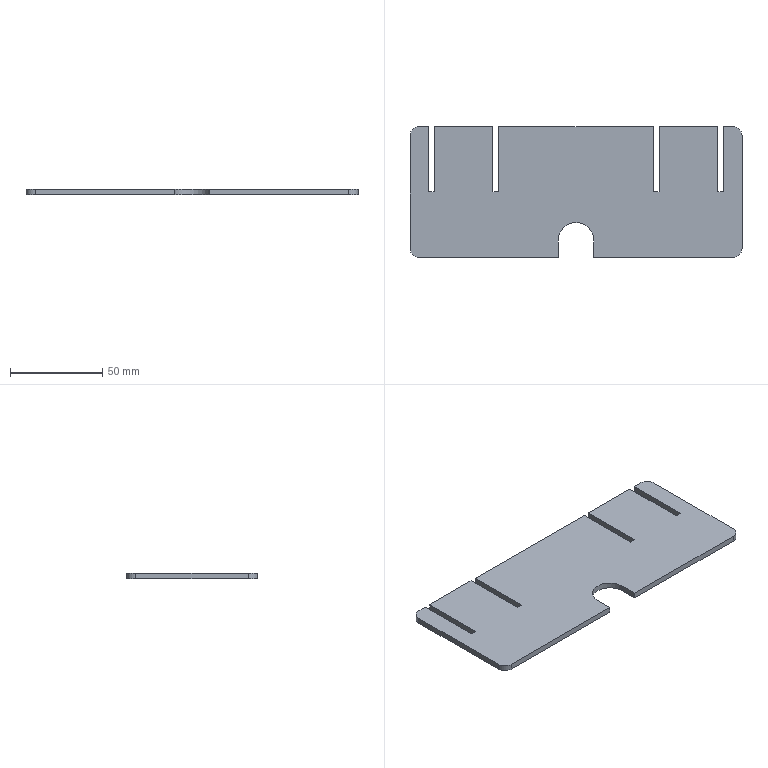Part | SolidWorks | features FlatPattern 1, SMBaseFlange 1, SheetMetal 1 | 1 solid | 30 faces | box 180 x 71 x 3.2 mm | volume 38342 mm3 | plane 25 | cylinder 5 | commonest cylinder face diameters 10 x4 19 x1
STEP:
#1=CARTESIAN_POINT('',(-146.71,-88.278,0.));
#2=VERTEX_POINT('',#1);
#3=CARTESIAN_POINT('',(-151.71,-88.278,0.));
#4=VERTEX_POINT('',#3);
#5=CARTESIAN_POINT('',(-146.71,-88.278,0.));
#6=DIRECTION('',(-1.,0.,0.));
#7=VECTOR('',#6,1000.);
#8=LINE('',#5,#7);
#9=EDGE_CURVE('',#2,#4,#8,.T.);
#10=ORIENTED_EDGE('',*,*,#9,.F.);
#11=CARTESIAN_POINT('',(-146.71,-88.278,-3.2));
#12=VERTEX_POINT('',#11);
#13=CARTESIAN_POINT('',(-146.71,-88.278,-3.2));
#14=DIRECTION('',(0.,0.,1.));
#15=VECTOR('',#14,1000.);
#16=LINE('',#13,#15);
#17=EDGE_CURVE('',#12,#2,#16,.T.);
#18=ORIENTED_EDGE('',*,*,#17,.F.);
#19=CARTESIAN_POINT('',(-151.71,-88.278,-3.2));
#20=VERTEX_POINT('',#19);
#21=CARTESIAN_POINT('',(-146.71,-88.278,-3.2));
#22=DIRECTION('',(-1.,0.,0.));
#23=VECTOR('',#22,1000.);
#24=LINE('',#21,#23);
#25=EDGE_CURVE('',#12,#20,#24,.T.);
#26=ORIENTED_EDGE('',*,*,#25,.T.);
#27=CARTESIAN_POINT('',(-151.71,-88.278,-3.2));
#28=DIRECTION('',(0.,0.,1.));
#29=VECTOR('',#28,1000.);
#30=LINE('',#27,#29);
#31=EDGE_CURVE('',#20,#4,#30,.T.);
#32=ORIENTED_EDGE('',*,*,#31,.T.);
#33=EDGE_LOOP('',(#10,#18,#26,#32));
#34=FACE_OUTER_BOUND('',#33,.T.);
#35=CARTESIAN_POINT('',(-146.71,-88.278,-3.2));
#36=DIRECTION('',(0.,1.,0.));
#37=DIRECTION('',(-1.,0.,0.));
#38=AXIS2_PLACEMENT_3D('',#35,#36,#37);
#39=PLANE('',#38);
#40=ADVANCED_FACE('',(#34),#39,.T.);
#41=CARTESIAN_POINT('',(-146.71,-123.778,0.));
#42=VERTEX_POINT('',#41);
#43=CARTESIAN_POINT('',(-146.71,-88.278,0.));
#44=DIRECTION('',(0.,1.,0.));
#45=VECTOR('',#44,1000.);
#46=LINE('',#43,#45);
#47=EDGE_CURVE('',#42,#2,#46,.T.);
#48=ORIENTED_EDGE('',*,*,#47,.F.);
#49=CARTESIAN_POINT('',(-146.71,-123.778,-3.2));
#50=VERTEX_POINT('',#49);
#51=CARTESIAN_POINT('',(-146.71,-123.778,-3.2));
#52=DIRECTION('',(0.,0.,1.));
#53=VECTOR('',#52,1000.);
#54=LINE('',#51,#53);
#55=EDGE_CURVE('',#50,#42,#54,.T.);
#56=ORIENTED_EDGE('',*,*,#55,.F.);
#57=CARTESIAN_POINT('',(-146.71,-88.278,-3.2));
#58=DIRECTION('',(0.,1.,0.));
#59=VECTOR('',#58,1000.);
#60=LINE('',#57,#59);
#61=EDGE_CURVE('',#50,#12,#60,.T.);
#62=ORIENTED_EDGE('',*,*,#61,.T.);
#63=ORIENTED_EDGE('',*,*,#17,.T.);
#64=EDGE_LOOP('',(#48,#56,#62,#63));
#65=FACE_OUTER_BOUND('',#64,.T.);
#66=CARTESIAN_POINT('',(-146.71,-88.278,-3.2));
#67=DIRECTION('',(1.,0.,0.));
#68=DIRECTION('',(0.,1.,0.));
#69=AXIS2_PLACEMENT_3D('',#66,#67,#68);
#70=PLANE('',#69);
#71=ADVANCED_FACE('',(#65),#70,.T.);
#72=CARTESIAN_POINT('',(-143.51,-123.778,0.));
#73=VERTEX_POINT('',#72);
#74=CARTESIAN_POINT('',(-146.71,-123.778,0.));
#75=DIRECTION('',(-1.,0.,0.));
#76=VECTOR('',#75,1000.);
#77=LINE('',#74,#76);
#78=EDGE_CURVE('',#73,#42,#77,.T.);
#79=ORIENTED_EDGE('',*,*,#78,.F.);
#80=CARTESIAN_POINT('',(-143.51,-123.778,-3.2));
#81=VERTEX_POINT('',#80);
#82=CARTESIAN_POINT('',(-143.51,-123.778,-3.2));
#83=DIRECTION('',(0.,0.,1.));
#84=VECTOR('',#83,1000.);
#85=LINE('',#82,#84);
#86=EDGE_CURVE('',#81,#73,#85,.T.);
#87=ORIENTED_EDGE('',*,*,#86,.F.);
#88=CARTESIAN_POINT('',(-146.71,-123.778,-3.2));
#89=DIRECTION('',(-1.,0.,0.));
#90=VECTOR('',#89,1000.);
#91=LINE('',#88,#90);
#92=EDGE_CURVE('',#81,#50,#91,.T.);
#93=ORIENTED_EDGE('',*,*,#92,.T.);
#94=ORIENTED_EDGE('',*,*,#55,.T.);
#95=EDGE_LOOP('',(#79,#87,#93,#94));
#96=FACE_OUTER_BOUND('',#95,.T.);
#97=CARTESIAN_POINT('',(-146.71,-123.778,-3.2));
#98=DIRECTION('',(0.,1.,0.));
#99=DIRECTION('',(0.,0.,1.));
#100=AXIS2_PLACEMENT_3D('',#97,#98,#99);
#101=PLANE('',#100);
#102=ADVANCED_FACE('',(#96),#101,.T.);
#103=CARTESIAN_POINT('',(-143.51,-88.278,0.));
#104=VERTEX_POINT('',#103);
#105=CARTESIAN_POINT('',(-143.51,-123.778,0.));
#106=DIRECTION('',(0.,-1.,0.));
#107=VECTOR('',#106,1000.);
#108=LINE('',#105,#107);
#109=EDGE_CURVE('',#104,#73,#108,.T.);
#110=ORIENTED_EDGE('',*,*,#109,.F.);
#111=CARTESIAN_POINT('',(-143.51,-88.278,-3.2));
#112=VERTEX_POINT('',#111);
#113=CARTESIAN_POINT('',(-143.51,-88.278,-3.2));
#114=DIRECTION('',(0.,0.,1.));
#115=VECTOR('',#114,1000.);
#116=LINE('',#113,#115);
#117=EDGE_CURVE('',#112,#104,#116,.T.);
#118=ORIENTED_EDGE('',*,*,#117,.F.);
#119=CARTESIAN_POINT('',(-143.51,-123.778,-3.2));
#120=DIRECTION('',(0.,-1.,0.));
#121=VECTOR('',#120,1000.);
#122=LINE('',#119,#121);
#123=EDGE_CURVE('',#112,#81,#122,.T.);
#124=ORIENTED_EDGE('',*,*,#123,.T.);
#125=ORIENTED_EDGE('',*,*,#86,.T.);
#126=EDGE_LOOP('',(#110,#118,#124,#125));
#127=FACE_OUTER_BOUND('',#126,.T.);
#128=CARTESIAN_POINT('',(-143.51,-123.778,-3.2));
#129=DIRECTION('',(-1.,0.,0.));
#130=DIRECTION('',(0.,-1.,0.));
#131=AXIS2_PLACEMENT_3D('',#128,#129,#130);
#132=PLANE('',#131);
#133=ADVANCED_FACE('',(#127),#132,.T.);
#134=CARTESIAN_POINT('',(-111.71,-88.278,0.));
#135=VERTEX_POINT('',#134);
#136=CARTESIAN_POINT('',(-111.71,-88.278,0.));
#137=DIRECTION('',(-1.,0.,0.));
#138=VECTOR('',#137,1000.);
#139=LINE('',#136,#138);
#140=EDGE_CURVE('',#135,#104,#139,.T.);
#141=ORIENTED_EDGE('',*,*,#140,.F.);
#142=CARTESIAN_POINT('',(-111.71,-88.278,-3.2));
#143=VERTEX_POINT('',#142);
#144=CARTESIAN_POINT('',(-111.71,-88.278,-3.2));
#145=DIRECTION('',(0.,0.,1.));
#146=VECTOR('',#145,1000.);
#147=LINE('',#144,#146);
#148=EDGE_CURVE('',#143,#135,#147,.T.);
#149=ORIENTED_EDGE('',*,*,#148,.F.);
#150=CARTESIAN_POINT('',(-111.71,-88.278,-3.2));
#151=DIRECTION('',(-1.,0.,0.));
#152=VECTOR('',#151,1000.);
#153=LINE('',#150,#152);
#154=EDGE_CURVE('',#143,#112,#153,.T.);
#155=ORIENTED_EDGE('',*,*,#154,.T.);
#156=ORIENTED_EDGE('',*,*,#117,.T.);
#157=EDGE_LOOP('',(#141,#149,#155,#156));
#158=FACE_OUTER_BOUND('',#157,.T.);
#159=CARTESIAN_POINT('',(-111.71,-88.278,-3.2));
#160=DIRECTION('',(0.,1.,0.));
#161=DIRECTION('',(-1.,0.,0.));
#162=AXIS2_PLACEMENT_3D('',#159,#160,#161);
#163=PLANE('',#162);
#164=ADVANCED_FACE('',(#158),#163,.T.);
#165=CARTESIAN_POINT('',(-111.71,-123.778,0.));
#166=VERTEX_POINT('',#165);
#167=CARTESIAN_POINT('',(-111.71,-88.278,0.));
#168=DIRECTION('',(0.,1.,0.));
#169=VECTOR('',#168,1000.);
#170=LINE('',#167,#169);
#171=EDGE_CURVE('',#166,#135,#170,.T.);
#172=ORIENTED_EDGE('',*,*,#171,.F.);
#173=CARTESIAN_POINT('',(-111.71,-123.778,-3.2));
#174=VERTEX_POINT('',#173);
#175=CARTESIAN_POINT('',(-111.71,-123.778,-3.2));
#176=DIRECTION('',(0.,0.,1.));
#177=VECTOR('',#176,1000.);
#178=LINE('',#175,#177);
#179=EDGE_CURVE('',#174,#166,#178,.T.);
#180=ORIENTED_EDGE('',*,*,#179,.F.);
#181=CARTESIAN_POINT('',(-111.71,-88.278,-3.2));
#182=DIRECTION('',(0.,1.,0.));
#183=VECTOR('',#182,1000.);
#184=LINE('',#181,#183);
#185=EDGE_CURVE('',#174,#143,#184,.T.);
#186=ORIENTED_EDGE('',*,*,#185,.T.);
#187=ORIENTED_EDGE('',*,*,#148,.T.);
#188=EDGE_LOOP('',(#172,#180,#186,#187));
#189=FACE_OUTER_BOUND('',#188,.T.);
#190=CARTESIAN_POINT('',(-111.71,-88.278,-3.2));
#191=DIRECTION('',(1.,0.,0.));
#192=DIRECTION('',(0.,1.,0.));
#193=AXIS2_PLACEMENT_3D('',#190,#191,#192);
#194=PLANE('',#193);
#195=ADVANCED_FACE('',(#189),#194,.T.);
#196=CARTESIAN_POINT('',(-108.51,-123.778,0.));
#197=VERTEX_POINT('',#196);
#198=CARTESIAN_POINT('',(-111.71,-123.778,0.));
#199=DIRECTION('',(-1.,0.,0.));
#200=VECTOR('',#199,1000.);
#201=LINE('',#198,#200);
#202=EDGE_CURVE('',#197,#166,#201,.T.);
#203=ORIENTED_EDGE('',*,*,#202,.F.);
#204=CARTESIAN_POINT('',(-108.51,-123.778,-3.2));
#205=VERTEX_POINT('',#204);
#206=CARTESIAN_POINT('',(-108.51,-123.778,-3.2));
#207=DIRECTION('',(0.,0.,1.));
#208=VECTOR('',#207,1000.);
#209=LINE('',#206,#208);
#210=EDGE_CURVE('',#205,#197,#209,.T.);
#211=ORIENTED_EDGE('',*,*,#210,.F.);
#212=CARTESIAN_POINT('',(-111.71,-123.778,-3.2));
#213=DIRECTION('',(-1.,0.,0.));
#214=VECTOR('',#213,1000.);
#215=LINE('',#212,#214);
#216=EDGE_CURVE('',#205,#174,#215,.T.);
#217=ORIENTED_EDGE('',*,*,#216,.T.);
#218=ORIENTED_EDGE('',*,*,#179,.T.);
#219=EDGE_LOOP('',(#203,#211,#217,#218));
#220=FACE_OUTER_BOUND('',#219,.T.);
#221=CARTESIAN_POINT('',(-111.71,-123.778,-3.2));
#222=DIRECTION('',(0.,1.,0.));
#223=DIRECTION('',(0.,0.,1.));
#224=AXIS2_PLACEMENT_3D('',#221,#222,#223);
#225=PLANE('',#224);
#226=ADVANCED_FACE('',(#220),#225,.T.);
#227=CARTESIAN_POINT('',(-108.51,-88.278,0.));
#228=VERTEX_POINT('',#227);
#229=CARTESIAN_POINT('',(-108.51,-123.778,0.));
#230=DIRECTION('',(0.,-1.,0.));
#231=VECTOR('',#230,1000.);
#232=LINE('',#229,#231);
#233=EDGE_CURVE('',#228,#197,#232,.T.);
#234=ORIENTED_EDGE('',*,*,#233,.F.);
#235=CARTESIAN_POINT('',(-108.51,-88.278,-3.2));
#236=VERTEX_POINT('',#235);
#237=CARTESIAN_POINT('',(-108.51,-88.278,-3.2));
#238=DIRECTION('',(0.,0.,1.));
#239=VECTOR('',#238,1000.);
#240=LINE('',#237,#239);
#241=EDGE_CURVE('',#236,#228,#240,.T.);
#242=ORIENTED_EDGE('',*,*,#241,.F.);
#243=CARTESIAN_POINT('',(-108.51,-123.778,-3.2));
#244=DIRECTION('',(0.,-1.,0.));
#245=VECTOR('',#244,1000.);
#246=LINE('',#243,#245);
#247=EDGE_CURVE('',#236,#205,#246,.T.);
#248=ORIENTED_EDGE('',*,*,#247,.T.);
#249=ORIENTED_EDGE('',*,*,#210,.T.);
#250=EDGE_LOOP('',(#234,#242,#248,#249));
#251=FACE_OUTER_BOUND('',#250,.T.);
#252=CARTESIAN_POINT('',(-108.51,-123.778,-3.2));
#253=DIRECTION('',(-1.,0.,0.));
#254=DIRECTION('',(0.,-1.,0.));
#255=AXIS2_PLACEMENT_3D('',#252,#253,#254);
#256=PLANE('',#255);
#257=ADVANCED_FACE('',(#251),#256,.T.);
#258=CARTESIAN_POINT('',(-24.91,-88.278,0.));
#259=VERTEX_POINT('',#258);
#260=CARTESIAN_POINT('',(-24.91,-88.278,0.));
#261=DIRECTION('',(-1.,0.,0.));
#262=VECTOR('',#261,1000.);
#263=LINE('',#260,#262);
#264=EDGE_CURVE('',#259,#228,#263,.T.);
#265=ORIENTED_EDGE('',*,*,#264,.F.);
#266=CARTESIAN_POINT('',(-24.91,-88.278,-3.2));
#267=VERTEX_POINT('',#266);
#268=CARTESIAN_POINT('',(-24.91,-88.278,-3.2));
#269=DIRECTION('',(0.,0.,1.));
#270=VECTOR('',#269,1000.);
#271=LINE('',#268,#270);
#272=EDGE_CURVE('',#267,#259,#271,.T.);
#273=ORIENTED_EDGE('',*,*,#272,.F.);
#274=CARTESIAN_POINT('',(-24.91,-88.278,-3.2));
#275=DIRECTION('',(-1.,0.,0.));
#276=VECTOR('',#275,1000.);
#277=LINE('',#274,#276);
#278=EDGE_CURVE('',#267,#236,#277,.T.);
#279=ORIENTED_EDGE('',*,*,#278,.T.);
#280=ORIENTED_EDGE('',*,*,#241,.T.);
#281=EDGE_LOOP('',(#265,#273,#279,#280));
#282=FACE_OUTER_BOUND('',#281,.T.);
#283=CARTESIAN_POINT('',(-24.91,-88.278,-3.2));
#284=DIRECTION('',(0.,1.,0.));
#285=DIRECTION('',(-1.,0.,0.));
#286=AXIS2_PLACEMENT_3D('',#283,#284,#285);
#287=PLANE('',#286);
#288=ADVANCED_FACE('',(#282),#287,.T.);
#289=CARTESIAN_POINT('',(-24.91,-123.778,0.));
#290=VERTEX_POINT('',#289);
#291=CARTESIAN_POINT('',(-24.91,-88.278,0.));
#292=DIRECTION('',(0.,1.,0.));
#293=VECTOR('',#292,1000.);
#294=LINE('',#291,#293);
#295=EDGE_CURVE('',#290,#259,#294,.T.);
#296=ORIENTED_EDGE('',*,*,#295,.F.);
#297=CARTESIAN_POINT('',(-24.91,-123.778,-3.2));
#298=VERTEX_POINT('',#297);
#299=CARTESIAN_POINT('',(-24.91,-123.778,-3.2));
#300=DIRECTION('',(0.,0.,1.));
#301=VECTOR('',#300,1000.);
#302=LINE('',#299,#301);
#303=EDGE_CURVE('',#298,#290,#302,.T.);
#304=ORIENTED_EDGE('',*,*,#303,.F.);
#305=CARTESIAN_POINT('',(-24.91,-88.278,-3.2));
#306=DIRECTION('',(0.,1.,0.));
#307=VECTOR('',#306,1000.);
#308=LINE('',#305,#307);
#309=EDGE_CURVE('',#298,#267,#308,.T.);
#310=ORIENTED_EDGE('',*,*,#309,.T.);
#311=ORIENTED_EDGE('',*,*,#272,.T.);
#312=EDGE_LOOP('',(#296,#304,#310,#311));
#313=FACE_OUTER_BOUND('',#312,.T.);
#314=CARTESIAN_POINT('',(-24.91,-88.278,-3.2));
#315=DIRECTION('',(1.,0.,0.));
#316=DIRECTION('',(0.,1.,0.));
#317=AXIS2_PLACEMENT_3D('',#314,#315,#316);
#318=PLANE('',#317);
#319=ADVANCED_FACE('',(#313),#318,.T.);
#320=CARTESIAN_POINT('',(-21.71,-123.778,0.));
#321=VERTEX_POINT('',#320);
#322=CARTESIAN_POINT('',(-24.91,-123.778,0.));
#323=DIRECTION('',(-1.,0.,0.));
#324=VECTOR('',#323,1000.);
#325=LINE('',#322,#324);
#326=EDGE_CURVE('',#321,#290,#325,.T.);
#327=ORIENTED_EDGE('',*,*,#326,.F.);
#328=CARTESIAN_POINT('',(-21.71,-123.778,-3.2));
#329=VERTEX_POINT('',#328);
#330=CARTESIAN_POINT('',(-21.71,-123.778,-3.2));
#331=DIRECTION('',(0.,0.,1.));
#332=VECTOR('',#331,1000.);
#333=LINE('',#330,#332);
#334=EDGE_CURVE('',#329,#321,#333,.T.);
#335=ORIENTED_EDGE('',*,*,#334,.F.);
#336=CARTESIAN_POINT('',(-24.91,-123.778,-3.2));
#337=DIRECTION('',(-1.,0.,0.));
#338=VECTOR('',#337,1000.);
#339=LINE('',#336,#338);
#340=EDGE_CURVE('',#329,#298,#339,.T.);
#341=ORIENTED_EDGE('',*,*,#340,.T.);
#342=ORIENTED_EDGE('',*,*,#303,.T.);
#343=EDGE_LOOP('',(#327,#335,#341,#342));
#344=FACE_OUTER_BOUND('',#343,.T.);
#345=CARTESIAN_POINT('',(-24.91,-123.778,-3.2));
#346=DIRECTION('',(0.,1.,0.));
#347=DIRECTION('',(0.,0.,1.));
#348=AXIS2_PLACEMENT_3D('',#345,#346,#347);
#349=PLANE('',#348);
#350=ADVANCED_FACE('',(#344),#349,.T.);
#351=CARTESIAN_POINT('',(-21.71,-88.278,0.));
#352=VERTEX_POINT('',#351);
#353=CARTESIAN_POINT('',(-21.71,-123.778,0.));
#354=DIRECTION('',(0.,-1.,0.));
#355=VECTOR('',#354,1000.);
#356=LINE('',#353,#355);
#357=EDGE_CURVE('',#352,#321,#356,.T.);
#358=ORIENTED_EDGE('',*,*,#357,.F.);
#359=CARTESIAN_POINT('',(-21.71,-88.278,-3.2));
#360=VERTEX_POINT('',#359);
#361=CARTESIAN_POINT('',(-21.71,-88.278,-3.2));
#362=DIRECTION('',(0.,0.,1.));
#363=VECTOR('',#362,1000.);
#364=LINE('',#361,#363);
#365=EDGE_CURVE('',#360,#352,#364,.T.);
#366=ORIENTED_EDGE('',*,*,#365,.F.);
#367=CARTESIAN_POINT('',(-21.71,-123.778,-3.2));
#368=DIRECTION('',(0.,-1.,0.));
#369=VECTOR('',#368,1000.);
#370=LINE('',#367,#369);
#371=EDGE_CURVE('',#360,#329,#370,.T.);
#372=ORIENTED_EDGE('',*,*,#371,.T.);
#373=ORIENTED_EDGE('',*,*,#334,.T.);
#374=EDGE_LOOP('',(#358,#366,#372,#373));
#375=FACE_OUTER_BOUND('',#374,.T.);
#376=CARTESIAN_POINT('',(-21.71,-123.778,-3.2));
#377=DIRECTION('',(-1.,0.,0.));
#378=DIRECTION('',(0.,-1.,0.));
#379=AXIS2_PLACEMENT_3D('',#376,#377,#378);
#380=PLANE('',#379);
#381=ADVANCED_FACE('',(#375),#380,.T.);
#382=CARTESIAN_POINT('',(10.09,-88.278,0.));
#383=VERTEX_POINT('',#382);
#384=CARTESIAN_POINT('',(10.09,-88.278,0.));
#385=DIRECTION('',(-1.,0.,0.));
#386=VECTOR('',#385,1000.);
#387=LINE('',#384,#386);
#388=EDGE_CURVE('',#383,#352,#387,.T.);
#389=ORIENTED_EDGE('',*,*,#388,.F.);
#390=CARTESIAN_POINT('',(10.09,-88.278,-3.2));
#391=VERTEX_POINT('',#390);
#392=CARTESIAN_POINT('',(10.09,-88.278,-3.2));
#393=DIRECTION('',(0.,0.,1.));
#394=VECTOR('',#393,1000.);
#395=LINE('',#392,#394);
#396=EDGE_CURVE('',#391,#383,#395,.T.);
#397=ORIENTED_EDGE('',*,*,#396,.F.);
#398=CARTESIAN_POINT('',(10.09,-88.278,-3.2));
#399=DIRECTION('',(-1.,0.,0.));
#400=VECTOR('',#399,1000.);
#401=LINE('',#398,#400);
#402=EDGE_CURVE('',#391,#360,#401,.T.);
#403=ORIENTED_EDGE('',*,*,#402,.T.);
#404=ORIENTED_EDGE('',*,*,#365,.T.);
#405=EDGE_LOOP('',(#389,#397,#403,#404));
#406=FACE_OUTER_BOUND('',#405,.T.);
#407=CARTESIAN_POINT('',(10.09,-88.278,-3.2));
#408=DIRECTION('',(0.,1.,0.));
#409=DIRECTION('',(-1.,0.,0.));
#410=AXIS2_PLACEMENT_3D('',#407,#408,#409);
#411=PLANE('',#410);
#412=ADVANCED_FACE('',(#406),#411,.T.);
#413=CARTESIAN_POINT('',(10.09,-123.778,0.));
#414=VERTEX_POINT('',#413);
#415=CARTESIAN_POINT('',(10.09,-88.278,0.));
#416=DIRECTION('',(0.,1.,0.));
#417=VECTOR('',#416,1000.);
#418=LINE('',#415,#417);
#419=EDGE_CURVE('',#414,#383,#418,.T.);
#420=ORIENTED_EDGE('',*,*,#419,.F.);
#421=CARTESIAN_POINT('',(10.09,-123.778,-3.2));
#422=VERTEX_POINT('',#421);
#423=CARTESIAN_POINT('',(10.09,-123.778,-3.2));
#424=DIRECTION('',(0.,0.,1.));
#425=VECTOR('',#424,1000.);
#426=LINE('',#423,#425);
#427=EDGE_CURVE('',#422,#414,#426,.T.);
#428=ORIENTED_EDGE('',*,*,#427,.F.);
#429=CARTESIAN_POINT('',(10.09,-88.278,-3.2));
#430=DIRECTION('',(0.,1.,0.));
#431=VECTOR('',#430,1000.);
#432=LINE('',#429,#431);
#433=EDGE_CURVE('',#422,#391,#432,.T.);
#434=ORIENTED_EDGE('',*,*,#433,.T.);
#435=ORIENTED_EDGE('',*,*,#396,.T.);
#436=EDGE_LOOP('',(#420,#428,#434,#435));
#437=FACE_OUTER_BOUND('',#436,.T.);
#438=CARTESIAN_POINT('',(10.09,-88.278,-3.2));
#439=DIRECTION('',(1.,0.,0.));
#440=DIRECTION('',(0.,1.,0.));
#441=AXIS2_PLACEMENT_3D('',#438,#439,#440);
#442=PLANE('',#441);
#443=ADVANCED_FACE('',(#437),#442,.T.);
#444=CARTESIAN_POINT('',(13.29,-123.778,0.));
#445=VERTEX_POINT('',#444);
#446=CARTESIAN_POINT('',(10.09,-123.778,0.));
#447=DIRECTION('',(-1.,0.,0.));
#448=VECTOR('',#447,1000.);
#449=LINE('',#446,#448);
#450=EDGE_CURVE('',#445,#414,#449,.T.);
#451=ORIENTED_EDGE('',*,*,#450,.F.);
#452=CARTESIAN_POINT('',(13.29,-123.778,-3.2));
#453=VERTEX_POINT('',#452);
#454=CARTESIAN_POINT('',(13.29,-123.778,-3.2));
#455=DIRECTION('',(0.,0.,1.));
#456=VECTOR('',#455,1000.);
#457=LINE('',#454,#456);
#458=EDGE_CURVE('',#453,#445,#457,.T.);
#459=ORIENTED_EDGE('',*,*,#458,.F.);
#460=CARTESIAN_POINT('',(10.09,-123.778,-3.2));
#461=DIRECTION('',(-1.,0.,0.));
#462=VECTOR('',#461,1000.);
#463=LINE('',#460,#462);
#464=EDGE_CURVE('',#453,#422,#463,.T.);
#465=ORIENTED_EDGE('',*,*,#464,.T.);
#466=ORIENTED_EDGE('',*,*,#427,.T.);
#467=EDGE_LOOP('',(#451,#459,#465,#466));
#468=FACE_OUTER_BOUND('',#467,.T.);
#469=CARTESIAN_POINT('',(10.09,-123.778,-3.2));
#470=DIRECTION('',(0.,1.,0.));
#471=DIRECTION('',(0.,0.,1.));
#472=AXIS2_PLACEMENT_3D('',#469,#470,#471);
#473=PLANE('',#472);
#474=ADVANCED_FACE('',(#468),#473,.T.);
#475=CARTESIAN_POINT('',(13.29,-88.278,0.));
#476=VERTEX_POINT('',#475);
#477=CARTESIAN_POINT('',(13.29,-123.778,0.));
#478=DIRECTION('',(0.,-1.,0.));
#479=VECTOR('',#478,1000.);
#480=LINE('',#477,#479);
#481=EDGE_CURVE('',#476,#445,#480,.T.);
#482=ORIENTED_EDGE('',*,*,#481,.F.);
#483=CARTESIAN_POINT('',(13.29,-88.278,-3.2));
#484=VERTEX_POINT('',#483);
#485=CARTESIAN_POINT('',(13.29,-88.278,-3.2));
#486=DIRECTION('',(0.,0.,1.));
#487=VECTOR('',#486,1000.);
#488=LINE('',#485,#487);
#489=EDGE_CURVE('',#484,#476,#488,.T.);
#490=ORIENTED_EDGE('',*,*,#489,.F.);
#491=CARTESIAN_POINT('',(13.29,-123.778,-3.2));
#492=DIRECTION('',(0.,-1.,0.));
#493=VECTOR('',#492,1000.);
#494=LINE('',#491,#493);
#495=EDGE_CURVE('',#484,#453,#494,.T.);
#496=ORIENTED_EDGE('',*,*,#495,.T.);
#497=ORIENTED_EDGE('',*,*,#458,.T.);
#498=EDGE_LOOP('',(#482,#490,#496,#497));
#499=FACE_OUTER_BOUND('',#498,.T.);
#500=CARTESIAN_POINT('',(13.29,-123.778,-3.2));
#501=DIRECTION('',(-1.,0.,0.));
#502=DIRECTION('',(0.,-1.,0.));
#503=AXIS2_PLACEMENT_3D('',#500,#501,#502);
#504=PLANE('',#503);
#505=ADVANCED_FACE('',(#499),#504,.T.);
#506=CARTESIAN_POINT('',(18.29,-88.278,0.));
#507=VERTEX_POINT('',#506);
#508=CARTESIAN_POINT('',(18.29,-88.278,0.));
#509=DIRECTION('',(-1.,0.,0.));
#510=VECTOR('',#509,1000.);
#511=LINE('',#508,#510);
#512=EDGE_CURVE('',#507,#476,#511,.T.);
#513=ORIENTED_EDGE('',*,*,#512,.F.);
#514=CARTESIAN_POINT('',(18.29,-88.278,-3.2));
#515=VERTEX_POINT('',#514);
#516=CARTESIAN_POINT('',(18.29,-88.278,-3.2));
#517=DIRECTION('',(0.,0.,1.));
#518=VECTOR('',#517,1000.);
#519=LINE('',#516,#518);
#520=EDGE_CURVE('',#515,#507,#519,.T.);
#521=ORIENTED_EDGE('',*,*,#520,.F.);
#522=CARTESIAN_POINT('',(18.29,-88.278,-3.2));
#523=DIRECTION('',(-1.,0.,0.));
#524=VECTOR('',#523,1000.);
#525=LINE('',#522,#524);
#526=EDGE_CURVE('',#515,#484,#525,.T.);
#527=ORIENTED_EDGE('',*,*,#526,.T.);
#528=ORIENTED_EDGE('',*,*,#489,.T.);
#529=EDGE_LOOP('',(#513,#521,#527,#528));
#530=FACE_OUTER_BOUND('',#529,.T.);
#531=CARTESIAN_POINT('',(18.29,-88.278,-3.2));
#532=DIRECTION('',(0.,1.,0.));
#533=DIRECTION('',(-1.,0.,0.));
#534=AXIS2_PLACEMENT_3D('',#531,#532,#533);
#535=PLANE('',#534);
#536=ADVANCED_FACE('',(#530),#535,.T.);
#537=CARTESIAN_POINT('',(23.29,-93.278,0.));
#538=VERTEX_POINT('',#537);
#539=CARTESIAN_POINT('',(18.29,-93.278,0.));
#540=DIRECTION('',(0.,0.,1.));
#541=DIRECTION('',(1.,0.,0.));
#542=AXIS2_PLACEMENT_3D('',#539,#540,#541);
#543=CIRCLE('',#542,5.);
#544=EDGE_CURVE('',#538,#507,#543,.T.);
#545=ORIENTED_EDGE('',*,*,#544,.F.);
#546=CARTESIAN_POINT('',(23.29,-93.278,-3.2));
#547=VERTEX_POINT('',#546);
#548=CARTESIAN_POINT('',(23.29,-93.278,-3.2));
#549=DIRECTION('',(0.,0.,1.));
#550=VECTOR('',#549,1000.);
#551=LINE('',#548,#550);
#552=EDGE_CURVE('',#547,#538,#551,.T.);
#553=ORIENTED_EDGE('',*,*,#552,.F.);
#554=CARTESIAN_POINT('',(18.29,-93.278,-3.2));
#555=DIRECTION('',(0.,0.,1.));
#556=DIRECTION('',(1.,0.,0.));
#557=AXIS2_PLACEMENT_3D('',#554,#555,#556);
#558=CIRCLE('',#557,5.);
#559=EDGE_CURVE('',#547,#515,#558,.T.);
#560=ORIENTED_EDGE('',*,*,#559,.T.);
#561=ORIENTED_EDGE('',*,*,#520,.T.);
#562=EDGE_LOOP('',(#545,#553,#560,#561));
#563=FACE_OUTER_BOUND('',#562,.T.);
#564=CARTESIAN_POINT('',(18.29,-93.278,-3.2));
#565=DIRECTION('',(0.,0.,1.));
#566=DIRECTION('',(1.,0.,0.));
#567=AXIS2_PLACEMENT_3D('',#564,#565,#566);
#568=CYLINDRICAL_SURFACE('',#567,5.);
#569=ADVANCED_FACE('',(#563),#568,.T.);
#570=CARTESIAN_POINT('',(23.29,-154.278,0.));
#571=VERTEX_POINT('',#570);
#572=CARTESIAN_POINT('',(23.29,-154.278,0.));
#573=DIRECTION('',(0.,1.,0.));
#574=VECTOR('',#573,1000.);
#575=LINE('',#572,#574);
#576=EDGE_CURVE('',#571,#538,#575,.T.);
#577=ORIENTED_EDGE('',*,*,#576,.F.);
#578=CARTESIAN_POINT('',(23.29,-154.278,-3.2));
#579=VERTEX_POINT('',#578);
#580=CARTESIAN_POINT('',(23.29,-154.278,-3.2));
#581=DIRECTION('',(0.,0.,1.));
#582=VECTOR('',#581,1000.);
#583=LINE('',#580,#582);
#584=EDGE_CURVE('',#579,#571,#583,.T.);
#585=ORIENTED_EDGE('',*,*,#584,.F.);
#586=CARTESIAN_POINT('',(23.29,-154.278,-3.2));
#587=DIRECTION('',(0.,1.,0.));
#588=VECTOR('',#587,1000.);
#589=LINE('',#586,#588);
#590=EDGE_CURVE('',#579,#547,#589,.T.);
#591=ORIENTED_EDGE('',*,*,#590,.T.);
#592=ORIENTED_EDGE('',*,*,#552,.T.);
#593=EDGE_LOOP('',(#577,#585,#591,#592));
#594=FACE_OUTER_BOUND('',#593,.T.);
#595=CARTESIAN_POINT('',(23.29,-154.278,-3.2));
#596=DIRECTION('',(1.,0.,0.));
#597=DIRECTION('',(0.,1.,0.));
#598=AXIS2_PLACEMENT_3D('',#595,#596,#597);
#599=PLANE('',#598);
#600=ADVANCED_FACE('',(#594),#599,.T.);
#601=CARTESIAN_POINT('',(18.29,-159.278,0.));
#602=VERTEX_POINT('',#601);
#603=CARTESIAN_POINT('',(18.29,-154.278,0.));
#604=DIRECTION('',(0.,0.,1.));
#605=DIRECTION('',(1.,0.,0.));
#606=AXIS2_PLACEMENT_3D('',#603,#604,#605);
#607=CIRCLE('',#606,5.);
#608=EDGE_CURVE('',#602,#571,#607,.T.);
#609=ORIENTED_EDGE('',*,*,#608,.F.);
#610=CARTESIAN_POINT('',(18.29,-159.278,-3.2));
#611=VERTEX_POINT('',#610);
#612=CARTESIAN_POINT('',(18.29,-159.278,-3.2));
#613=DIRECTION('',(0.,0.,1.));
#614=VECTOR('',#613,1000.);
#615=LINE('',#612,#614);
#616=EDGE_CURVE('',#611,#602,#615,.T.);
#617=ORIENTED_EDGE('',*,*,#616,.F.);
#618=CARTESIAN_POINT('',(18.29,-154.278,-3.2));
#619=DIRECTION('',(0.,0.,1.));
#620=DIRECTION('',(1.,0.,0.));
#621=AXIS2_PLACEMENT_3D('',#618,#619,#620);
#622=CIRCLE('',#621,5.);
#623=EDGE_CURVE('',#611,#579,#622,.T.);
#624=ORIENTED_EDGE('',*,*,#623,.T.);
#625=ORIENTED_EDGE('',*,*,#584,.T.);
#626=EDGE_LOOP('',(#609,#617,#624,#625));
#627=FACE_OUTER_BOUND('',#626,.T.);
#628=CARTESIAN_POINT('',(18.29,-154.278,-3.2));
#629=DIRECTION('',(0.,0.,1.));
#630=DIRECTION('',(1.,0.,0.));
#631=AXIS2_PLACEMENT_3D('',#628,#629,#630);
#632=CYLINDRICAL_SURFACE('',#631,5.);
#633=ADVANCED_FACE('',(#627),#632,.T.);
#634=CARTESIAN_POINT('',(-57.21,-159.278,0.));
#635=VERTEX_POINT('',#634);
#636=CARTESIAN_POINT('',(-57.21,-159.278,0.));
#637=DIRECTION('',(1.,0.,0.));
#638=VECTOR('',#637,1000.);
#639=LINE('',#636,#638);
#640=EDGE_CURVE('',#635,#602,#639,.T.);
#641=ORIENTED_EDGE('',*,*,#640,.F.);
#642=CARTESIAN_POINT('',(-57.21,-159.278,-3.2));
#643=VERTEX_POINT('',#642);
#644=CARTESIAN_POINT('',(-57.21,-159.278,-3.2));
#645=DIRECTION('',(0.,0.,1.));
#646=VECTOR('',#645,1000.);
#647=LINE('',#644,#646);
#648=EDGE_CURVE('',#643,#635,#647,.T.);
#649=ORIENTED_EDGE('',*,*,#648,.F.);
#650=CARTESIAN_POINT('',(-57.21,-159.278,-3.2));
#651=DIRECTION('',(1.,0.,0.));
#652=VECTOR('',#651,1000.);
#653=LINE('',#650,#652);
#654=EDGE_CURVE('',#643,#611,#653,.T.);
#655=ORIENTED_EDGE('',*,*,#654,.T.);
#656=ORIENTED_EDGE('',*,*,#616,.T.);
#657=EDGE_LOOP('',(#641,#649,#655,#656));
#658=FACE_OUTER_BOUND('',#657,.T.);
#659=CARTESIAN_POINT('',(-57.21,-159.278,-3.2));
#660=DIRECTION('',(0.,-1.,0.));
#661=DIRECTION('',(0.,0.,-1.));
#662=AXIS2_PLACEMENT_3D('',#659,#660,#661);
#663=PLANE('',#662);
#664=ADVANCED_FACE('',(#658),#663,.T.);
#665=CARTESIAN_POINT('',(-57.21,-149.778,0.));
#666=VERTEX_POINT('',#665);
#667=CARTESIAN_POINT('',(-57.21,-149.778,0.));
#668=DIRECTION('',(0.,-1.,0.));
#669=VECTOR('',#668,1000.);
#670=LINE('',#667,#669);
#671=EDGE_CURVE('',#666,#635,#670,.T.);
#672=ORIENTED_EDGE('',*,*,#671,.F.);
#673=CARTESIAN_POINT('',(-57.21,-149.778,-3.2));
#674=VERTEX_POINT('',#673);
#675=CARTESIAN_POINT('',(-57.21,-149.778,-3.2));
#676=DIRECTION('',(0.,0.,1.));
#677=VECTOR('',#676,1000.);
#678=LINE('',#675,#677);
#679=EDGE_CURVE('',#674,#666,#678,.T.);
#680=ORIENTED_EDGE('',*,*,#679,.F.);
#681=CARTESIAN_POINT('',(-57.21,-149.778,-3.2));
#682=DIRECTION('',(0.,-1.,0.));
#683=VECTOR('',#682,1000.);
#684=LINE('',#681,#683);
#685=EDGE_CURVE('',#674,#643,#684,.T.);
#686=ORIENTED_EDGE('',*,*,#685,.T.);
#687=ORIENTED_EDGE('',*,*,#648,.T.);
#688=EDGE_LOOP('',(#672,#680,#686,#687));
#689=FACE_OUTER_BOUND('',#688,.T.);
#690=CARTESIAN_POINT('',(-57.21,-149.778,-3.2));
#691=DIRECTION('',(-1.,0.,0.));
#692=DIRECTION('',(0.,-1.,0.));
#693=AXIS2_PLACEMENT_3D('',#690,#691,#692);
#694=PLANE('',#693);
#695=ADVANCED_FACE('',(#689),#694,.T.);
#696=CARTESIAN_POINT('',(-76.21,-149.778,0.));
#697=VERTEX_POINT('',#696);
#698=CARTESIAN_POINT('',(-66.71,-149.778,0.));
#699=DIRECTION('',(0.,0.,-1.));
#700=DIRECTION('',(1.,0.,0.));
#701=AXIS2_PLACEMENT_3D('',#698,#699,#700);
#702=CIRCLE('',#701,9.5);
#703=EDGE_CURVE('',#697,#666,#702,.T.);
#704=ORIENTED_EDGE('',*,*,#703,.F.);
#705=CARTESIAN_POINT('',(-76.21,-149.778,-3.2));
#706=VERTEX_POINT('',#705);
#707=CARTESIAN_POINT('',(-76.21,-149.778,-3.2));
#708=DIRECTION('',(0.,0.,1.));
#709=VECTOR('',#708,1000.);
#710=LINE('',#707,#709);
#711=EDGE_CURVE('',#706,#697,#710,.T.);
#712=ORIENTED_EDGE('',*,*,#711,.F.);
#713=CARTESIAN_POINT('',(-66.71,-149.778,-3.2));
#714=DIRECTION('',(0.,0.,-1.));
#715=DIRECTION('',(1.,0.,0.));
#716=AXIS2_PLACEMENT_3D('',#713,#714,#715);
#717=CIRCLE('',#716,9.5);
#718=EDGE_CURVE('',#706,#674,#717,.T.);
#719=ORIENTED_EDGE('',*,*,#718,.T.);
#720=ORIENTED_EDGE('',*,*,#679,.T.);
#721=EDGE_LOOP('',(#704,#712,#719,#720));
#722=FACE_OUTER_BOUND('',#721,.T.);
#723=CARTESIAN_POINT('',(-66.71,-149.778,-3.2));
#724=DIRECTION('',(0.,0.,1.));
#725=DIRECTION('',(1.,0.,0.));
#726=AXIS2_PLACEMENT_3D('',#723,#724,#725);
#727=CYLINDRICAL_SURFACE('',#726,9.5);
#728=ADVANCED_FACE('',(#722),#727,.F.);
#729=CARTESIAN_POINT('',(-76.21,-159.278,0.));
#730=VERTEX_POINT('',#729);
#731=CARTESIAN_POINT('',(-76.21,-159.278,0.));
#732=DIRECTION('',(0.,1.,0.));
#733=VECTOR('',#732,1000.);
#734=LINE('',#731,#733);
#735=EDGE_CURVE('',#730,#697,#734,.T.);
#736=ORIENTED_EDGE('',*,*,#735,.F.);
#737=CARTESIAN_POINT('',(-76.21,-159.278,-3.2));
#738=VERTEX_POINT('',#737);
#739=CARTESIAN_POINT('',(-76.21,-159.278,-3.2));
#740=DIRECTION('',(0.,0.,1.));
#741=VECTOR('',#740,1000.);
#742=LINE('',#739,#741);
#743=EDGE_CURVE('',#738,#730,#742,.T.);
#744=ORIENTED_EDGE('',*,*,#743,.F.);
#745=CARTESIAN_POINT('',(-76.21,-159.278,-3.2));
#746=DIRECTION('',(0.,1.,0.));
#747=VECTOR('',#746,1000.);
#748=LINE('',#745,#747);
#749=EDGE_CURVE('',#738,#706,#748,.T.);
#750=ORIENTED_EDGE('',*,*,#749,.T.);
#751=ORIENTED_EDGE('',*,*,#711,.T.);
#752=EDGE_LOOP('',(#736,#744,#750,#751));
#753=FACE_OUTER_BOUND('',#752,.T.);
#754=CARTESIAN_POINT('',(-76.21,-159.278,-3.2));
#755=DIRECTION('',(1.,0.,0.));
#756=DIRECTION('',(0.,0.,-1.));
#757=AXIS2_PLACEMENT_3D('',#754,#755,#756);
#758=PLANE('',#757);
#759=ADVANCED_FACE('',(#753),#758,.T.);
#760=CARTESIAN_POINT('',(-151.71,-159.278,0.));
#761=VERTEX_POINT('',#760);
#762=CARTESIAN_POINT('',(-151.71,-159.278,0.));
#763=DIRECTION('',(1.,0.,0.));
#764=VECTOR('',#763,1000.);
#765=LINE('',#762,#764);
#766=EDGE_CURVE('',#761,#730,#765,.T.);
#767=ORIENTED_EDGE('',*,*,#766,.F.);
#768=CARTESIAN_POINT('',(-151.71,-159.278,-3.2));
#769=VERTEX_POINT('',#768);
#770=CARTESIAN_POINT('',(-151.71,-159.278,-3.2));
#771=DIRECTION('',(0.,0.,1.));
#772=VECTOR('',#771,1000.);
#773=LINE('',#770,#772);
#774=EDGE_CURVE('',#769,#761,#773,.T.);
#775=ORIENTED_EDGE('',*,*,#774,.F.);
#776=CARTESIAN_POINT('',(-151.71,-159.278,-3.2));
#777=DIRECTION('',(1.,0.,0.));
#778=VECTOR('',#777,1000.);
#779=LINE('',#776,#778);
#780=EDGE_CURVE('',#769,#738,#779,.T.);
#781=ORIENTED_EDGE('',*,*,#780,.T.);
#782=ORIENTED_EDGE('',*,*,#743,.T.);
#783=EDGE_LOOP('',(#767,#775,#781,#782));
#784=FACE_OUTER_BOUND('',#783,.T.);
#785=CARTESIAN_POINT('',(-151.71,-159.278,-3.2));
#786=DIRECTION('',(0.,-1.,0.));
#787=DIRECTION('',(0.,0.,-1.));
#788=AXIS2_PLACEMENT_3D('',#785,#786,#787);
#789=PLANE('',#788);
#790=ADVANCED_FACE('',(#784),#789,.T.);
#791=CARTESIAN_POINT('',(-156.71,-154.278,0.));
#792=VERTEX_POINT('',#791);
#793=CARTESIAN_POINT('',(-151.71,-154.278,0.));
#794=DIRECTION('',(0.,0.,1.));
#795=DIRECTION('',(1.,0.,0.));
#796=AXIS2_PLACEMENT_3D('',#793,#794,#795);
#797=CIRCLE('',#796,5.);
#798=EDGE_CURVE('',#792,#761,#797,.T.);
#799=ORIENTED_EDGE('',*,*,#798,.F.);
#800=CARTESIAN_POINT('',(-156.71,-154.278,-3.2));
#801=VERTEX_POINT('',#800);
#802=CARTESIAN_POINT('',(-156.71,-154.278,-3.2));
#803=DIRECTION('',(0.,0.,1.));
#804=VECTOR('',#803,1000.);
#805=LINE('',#802,#804);
#806=EDGE_CURVE('',#801,#792,#805,.T.);
#807=ORIENTED_EDGE('',*,*,#806,.F.);
#808=CARTESIAN_POINT('',(-151.71,-154.278,-3.2));
#809=DIRECTION('',(0.,0.,1.));
#810=DIRECTION('',(1.,0.,0.));
#811=AXIS2_PLACEMENT_3D('',#808,#809,#810);
#812=CIRCLE('',#811,5.);
#813=EDGE_CURVE('',#801,#769,#812,.T.);
#814=ORIENTED_EDGE('',*,*,#813,.T.);
#815=ORIENTED_EDGE('',*,*,#774,.T.);
#816=EDGE_LOOP('',(#799,#807,#814,#815));
#817=FACE_OUTER_BOUND('',#816,.T.);
#818=CARTESIAN_POINT('',(-151.71,-154.278,-3.2));
#819=DIRECTION('',(0.,0.,1.));
#820=DIRECTION('',(1.,0.,0.));
#821=AXIS2_PLACEMENT_3D('',#818,#819,#820);
#822=CYLINDRICAL_SURFACE('',#821,5.);
#823=ADVANCED_FACE('',(#817),#822,.T.);
#824=CARTESIAN_POINT('',(-156.71,-93.278,0.));
#825=VERTEX_POINT('',#824);
#826=CARTESIAN_POINT('',(-156.71,-93.278,0.));
#827=DIRECTION('',(0.,-1.,0.));
#828=VECTOR('',#827,1000.);
#829=LINE('',#826,#828);
#830=EDGE_CURVE('',#825,#792,#829,.T.);
#831=ORIENTED_EDGE('',*,*,#830,.F.);
#832=CARTESIAN_POINT('',(-156.71,-93.278,-3.2));
#833=VERTEX_POINT('',#832);
#834=CARTESIAN_POINT('',(-156.71,-93.278,-3.2));
#835=DIRECTION('',(0.,0.,1.));
#836=VECTOR('',#835,1000.);
#837=LINE('',#834,#836);
#838=EDGE_CURVE('',#833,#825,#837,.T.);
#839=ORIENTED_EDGE('',*,*,#838,.F.);
#840=CARTESIAN_POINT('',(-156.71,-93.278,-3.2));
#841=DIRECTION('',(0.,-1.,0.));
#842=VECTOR('',#841,1000.);
#843=LINE('',#840,#842);
#844=EDGE_CURVE('',#833,#801,#843,.T.);
#845=ORIENTED_EDGE('',*,*,#844,.T.);
#846=ORIENTED_EDGE('',*,*,#806,.T.);
#847=EDGE_LOOP('',(#831,#839,#845,#846));
#848=FACE_OUTER_BOUND('',#847,.T.);
#849=CARTESIAN_POINT('',(-156.71,-93.278,-3.2));
#850=DIRECTION('',(-1.,0.,0.));
#851=DIRECTION('',(0.,0.,1.));
#852=AXIS2_PLACEMENT_3D('',#849,#850,#851);
#853=PLANE('',#852);
#854=ADVANCED_FACE('',(#848),#853,.T.);
#855=CARTESIAN_POINT('',(-151.71,-93.278,0.));
#856=DIRECTION('',(0.,0.,1.));
#857=DIRECTION('',(1.,0.,0.));
#858=AXIS2_PLACEMENT_3D('',#855,#856,#857);
#859=CIRCLE('',#858,5.);
#860=EDGE_CURVE('',#4,#825,#859,.T.);
#861=ORIENTED_EDGE('',*,*,#860,.F.);
#862=ORIENTED_EDGE('',*,*,#31,.F.);
#863=CARTESIAN_POINT('',(-151.71,-93.278,-3.2));
#864=DIRECTION('',(0.,0.,1.));
#865=DIRECTION('',(1.,0.,0.));
#866=AXIS2_PLACEMENT_3D('',#863,#864,#865);
#867=CIRCLE('',#866,5.);
#868=EDGE_CURVE('',#20,#833,#867,.T.);
#869=ORIENTED_EDGE('',*,*,#868,.T.);
#870=ORIENTED_EDGE('',*,*,#838,.T.);
#871=EDGE_LOOP('',(#861,#862,#869,#870));
#872=FACE_OUTER_BOUND('',#871,.T.);
#873=CARTESIAN_POINT('',(-151.71,-93.278,-3.2));
#874=DIRECTION('',(0.,0.,1.));
#875=DIRECTION('',(1.,0.,0.));
#876=AXIS2_PLACEMENT_3D('',#873,#874,#875);
#877=CYLINDRICAL_SURFACE('',#876,5.);
#878=ADVANCED_FACE('',(#872),#877,.T.);
#879=ORIENTED_EDGE('',*,*,#25,.F.);
#880=ORIENTED_EDGE('',*,*,#61,.F.);
#881=ORIENTED_EDGE('',*,*,#92,.F.);
#882=ORIENTED_EDGE('',*,*,#123,.F.);
#883=ORIENTED_EDGE('',*,*,#154,.F.);
#884=ORIENTED_EDGE('',*,*,#185,.F.);
#885=ORIENTED_EDGE('',*,*,#216,.F.);
#886=ORIENTED_EDGE('',*,*,#247,.F.);
#887=ORIENTED_EDGE('',*,*,#278,.F.);
#888=ORIENTED_EDGE('',*,*,#309,.F.);
#889=ORIENTED_EDGE('',*,*,#340,.F.);
#890=ORIENTED_EDGE('',*,*,#371,.F.);
#891=ORIENTED_EDGE('',*,*,#402,.F.);
#892=ORIENTED_EDGE('',*,*,#433,.F.);
#893=ORIENTED_EDGE('',*,*,#464,.F.);
#894=ORIENTED_EDGE('',*,*,#495,.F.);
#895=ORIENTED_EDGE('',*,*,#526,.F.);
#896=ORIENTED_EDGE('',*,*,#559,.F.);
#897=ORIENTED_EDGE('',*,*,#590,.F.);
#898=ORIENTED_EDGE('',*,*,#623,.F.);
#899=ORIENTED_EDGE('',*,*,#654,.F.);
#900=ORIENTED_EDGE('',*,*,#685,.F.);
#901=ORIENTED_EDGE('',*,*,#718,.F.);
#902=ORIENTED_EDGE('',*,*,#749,.F.);
#903=ORIENTED_EDGE('',*,*,#780,.F.);
#904=ORIENTED_EDGE('',*,*,#813,.F.);
#905=ORIENTED_EDGE('',*,*,#844,.F.);
#906=ORIENTED_EDGE('',*,*,#868,.F.);
#907=EDGE_LOOP('',(#879,#880,#881,#882,#883,#884,#885,#886,#887,#888,#889,#890,#891,#892,#893,#894,#895,#896,#897,#898,#899,#900,#901,#902,#903,#904,#905,#906));
#908=FACE_OUTER_BOUND('',#907,.T.);
#909=CARTESIAN_POINT('',(-151.71,-93.278,-3.2));
#910=DIRECTION('',(0.,0.,1.));
#911=DIRECTION('',(1.,0.,0.));
#912=AXIS2_PLACEMENT_3D('',#909,#910,#911);
#913=PLANE('',#912);
#914=ADVANCED_FACE('',(#908),#913,.F.);
#915=ORIENTED_EDGE('',*,*,#9,.T.);
#916=ORIENTED_EDGE('',*,*,#860,.T.);
#917=ORIENTED_EDGE('',*,*,#830,.T.);
#918=ORIENTED_EDGE('',*,*,#798,.T.);
#919=ORIENTED_EDGE('',*,*,#766,.T.);
#920=ORIENTED_EDGE('',*,*,#735,.T.);
#921=ORIENTED_EDGE('',*,*,#703,.T.);
#922=ORIENTED_EDGE('',*,*,#671,.T.);
#923=ORIENTED_EDGE('',*,*,#640,.T.);
#924=ORIENTED_EDGE('',*,*,#608,.T.);
#925=ORIENTED_EDGE('',*,*,#576,.T.);
#926=ORIENTED_EDGE('',*,*,#544,.T.);
#927=ORIENTED_EDGE('',*,*,#512,.T.);
#928=ORIENTED_EDGE('',*,*,#481,.T.);
#929=ORIENTED_EDGE('',*,*,#450,.T.);
#930=ORIENTED_EDGE('',*,*,#419,.T.);
#931=ORIENTED_EDGE('',*,*,#388,.T.);
#932=ORIENTED_EDGE('',*,*,#357,.T.);
#933=ORIENTED_EDGE('',*,*,#326,.T.);
#934=ORIENTED_EDGE('',*,*,#295,.T.);
#935=ORIENTED_EDGE('',*,*,#264,.T.);
#936=ORIENTED_EDGE('',*,*,#233,.T.);
#937=ORIENTED_EDGE('',*,*,#202,.T.);
#938=ORIENTED_EDGE('',*,*,#171,.T.);
#939=ORIENTED_EDGE('',*,*,#140,.T.);
#940=ORIENTED_EDGE('',*,*,#109,.T.);
#941=ORIENTED_EDGE('',*,*,#78,.T.);
#942=ORIENTED_EDGE('',*,*,#47,.T.);
#943=EDGE_LOOP('',(#915,#916,#917,#918,#919,#920,#921,#922,#923,#924,#925,#926,#927,#928,#929,#930,#931,#932,#933,#934,#935,#936,#937,#938,#939,#940,#941,#942));
#944=FACE_OUTER_BOUND('',#943,.T.);
#945=CARTESIAN_POINT('',(-151.71,-93.278,0.));
#946=DIRECTION('',(0.,0.,1.));
#947=DIRECTION('',(1.,0.,0.));
#948=AXIS2_PLACEMENT_3D('',#945,#946,#947);
#949=PLANE('',#948);
#950=ADVANCED_FACE('',(#944),#949,.T.);
#951=CLOSED_SHELL('',(#40,#71,#102,#133,#164,#195,#226,#257,#288,#319,#350,#381,#412,#443,#474,#505,#536,#569,#600,#633,#664,#695,#728,#759,#790,#823,#854,#878,#914,#950));
#952=MANIFOLD_SOLID_BREP('',#951);
#953=CARTESIAN_POINT('',(0.,0.,0.));
#954=DIRECTION('',(0.,0.,1.));
#955=DIRECTION('',(1.,0.,0.));
#956=AXIS2_PLACEMENT_3D('',#953,#954,#955);
#957=(LENGTH_UNIT()NAMED_UNIT(*)SI_UNIT(.MILLI.,.METRE.));
#958=UNCERTAINTY_MEASURE_WITH_UNIT(LENGTH_MEASURE(0.00001),#957,'','');
#959=(NAMED_UNIT(*)PLANE_ANGLE_UNIT()SI_UNIT($,.RADIAN.));
#960=(NAMED_UNIT(*)SI_UNIT($,.STERADIAN.)SOLID_ANGLE_UNIT());
#961=(GEOMETRIC_REPRESENTATION_CONTEXT(3)GLOBAL_UNCERTAINTY_ASSIGNED_CONTEXT((#958))GLOBAL_UNIT_ASSIGNED_CONTEXT((#957,#959,#960))REPRESENTATION_CONTEXT('',''));
#962=ADVANCED_BREP_SHAPE_REPRESENTATION('',(#952,#956),#961);